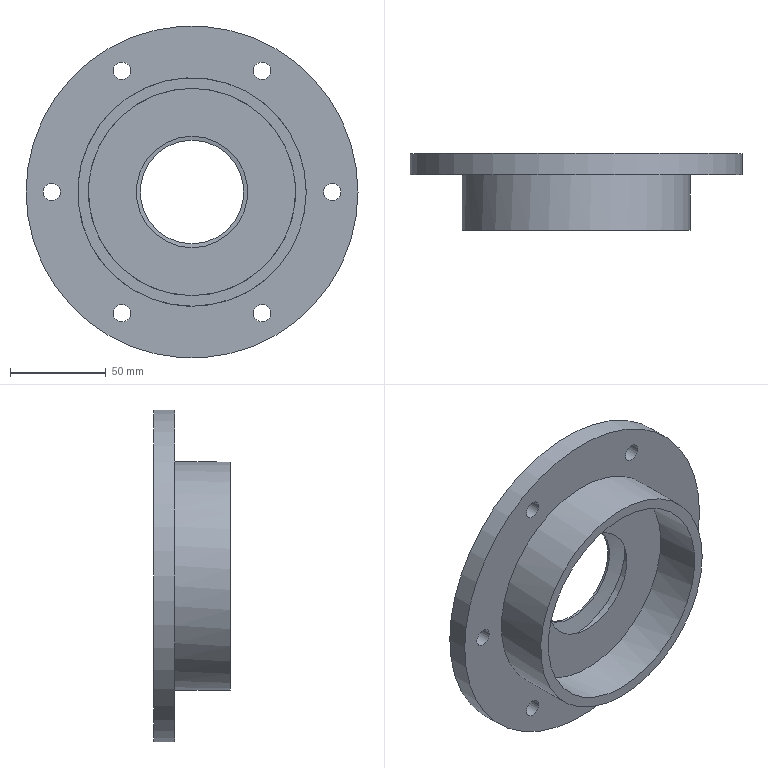Part | NX | features DATUM_CSYS 10, HOLE PACKAGE 10, SIMPLE HOLE 10, SKETCH 9, EXTRACT_DATUM_AXIS 6, EXTRACT_FACE 6, Instance Feature 5, EXTRUDE 2, DELETE FACE 1, OFFSET_REGION 1, Pattern Feature 1, SWP104 1 | 1 solid | 19 faces | box 173 x 40 x 173 mm | volume 270737 mm3 | cylinder 12 | plane 5 | cone 2 | commonest cylinder face diameters 9 x6 54 x1 74 x1 108 x1 114 x1 119 x1
STEP:
#1=CARTESIAN_POINT('',(0.,-15.,54.));
#2=VERTEX_POINT('',#1);
#3=CARTESIAN_POINT('',(0.,-15.,0.));
#4=DIRECTION('',(0.,1.,0.));
#5=DIRECTION('',(0.,0.,1.));
#6=AXIS2_PLACEMENT_3D('',#3,#4,#5);
#7=CIRCLE('',#6,54.);
#8=EDGE_CURVE('',#2,#2,#7,.F.);
#9=ORIENTED_EDGE('',*,*,#8,.T.);
#10=EDGE_LOOP('',(#9));
#11=FACE_BOUND('',#10,.T.);
#12=CARTESIAN_POINT('',(0.,-15.,29.059));
#13=VERTEX_POINT('',#12);
#14=CARTESIAN_POINT('',(0.,-15.,0.));
#15=DIRECTION('',(0.,1.,0.));
#16=DIRECTION('',(0.,0.,1.));
#17=AXIS2_PLACEMENT_3D('',#14,#15,#16);
#18=CIRCLE('',#17,29.059);
#19=EDGE_CURVE('',#13,#13,#18,.F.);
#20=ORIENTED_EDGE('',*,*,#19,.F.);
#21=EDGE_LOOP('',(#20));
#22=FACE_BOUND('',#21,.T.);
#23=CARTESIAN_POINT('',(0.,-15.,0.));
#24=DIRECTION('',(0.,1.,0.));
#25=DIRECTION('',(0.,0.,1.));
#26=AXIS2_PLACEMENT_3D('',#23,#24,#25);
#27=PLANE('',#26);
#28=ADVANCED_FACE('',(#11,#22),#27,.F.);
#29=CARTESIAN_POINT('',(86.5,-11.,0.));
#30=VERTEX_POINT('',#29);
#31=CARTESIAN_POINT('',(0.,-11.,0.));
#32=DIRECTION('',(0.,-1.,0.));
#33=DIRECTION('',(1.,0.,0.));
#34=AXIS2_PLACEMENT_3D('',#31,#32,#33);
#35=CIRCLE('',#34,86.5);
#36=EDGE_CURVE('',#30,#30,#35,.T.);
#37=ORIENTED_EDGE('',*,*,#36,.F.);
#38=EDGE_LOOP('',(#37));
#39=FACE_BOUND('',#38,.T.);
#40=CARTESIAN_POINT('',(86.5,0.,0.));
#41=VERTEX_POINT('',#40);
#42=CARTESIAN_POINT('',(0.,0.,0.));
#43=DIRECTION('',(0.,-1.,0.));
#44=DIRECTION('',(1.,0.,0.));
#45=AXIS2_PLACEMENT_3D('',#42,#43,#44);
#46=CIRCLE('',#45,86.5);
#47=EDGE_CURVE('',#41,#41,#46,.T.);
#48=ORIENTED_EDGE('',*,*,#47,.T.);
#49=EDGE_LOOP('',(#48));
#50=FACE_BOUND('',#49,.T.);
#51=CARTESIAN_POINT('',(0.,-11.,0.));
#52=DIRECTION('',(0.,1.,0.));
#53=DIRECTION('',(0.,0.,1.));
#54=AXIS2_PLACEMENT_3D('',#51,#52,#53);
#55=CYLINDRICAL_SURFACE('',#54,86.5);
#56=ADVANCED_FACE('',(#39,#50),#55,.T.);
#57=CARTESIAN_POINT('',(-36.5,-11.,-67.72));
#58=VERTEX_POINT('',#57);
#59=CARTESIAN_POINT('',(-36.5,-11.,-63.22));
#60=DIRECTION('',(0.,-1.,0.));
#61=DIRECTION('',(0.,0.,-1.));
#62=AXIS2_PLACEMENT_3D('',#59,#60,#61);
#63=CIRCLE('',#62,4.5);
#64=EDGE_CURVE('',#58,#58,#63,.T.);
#65=ORIENTED_EDGE('',*,*,#64,.F.);
#66=EDGE_LOOP('',(#65));
#67=FACE_BOUND('',#66,.T.);
#68=CARTESIAN_POINT('',(36.5,-11.,-67.72));
#69=VERTEX_POINT('',#68);
#70=CARTESIAN_POINT('',(36.5,-11.,-63.22));
#71=DIRECTION('',(0.,-1.,0.));
#72=DIRECTION('',(0.,0.,-1.));
#73=AXIS2_PLACEMENT_3D('',#70,#71,#72);
#74=CIRCLE('',#73,4.5);
#75=EDGE_CURVE('',#69,#69,#74,.T.);
#76=ORIENTED_EDGE('',*,*,#75,.F.);
#77=EDGE_LOOP('',(#76));
#78=FACE_BOUND('',#77,.T.);
#79=CARTESIAN_POINT('',(73.,-11.,-4.5));
#80=VERTEX_POINT('',#79);
#81=CARTESIAN_POINT('',(73.,-11.,0.));
#82=DIRECTION('',(0.,-1.,0.));
#83=DIRECTION('',(0.,0.,-1.));
#84=AXIS2_PLACEMENT_3D('',#81,#82,#83);
#85=CIRCLE('',#84,4.5);
#86=EDGE_CURVE('',#80,#80,#85,.T.);
#87=ORIENTED_EDGE('',*,*,#86,.F.);
#88=EDGE_LOOP('',(#87));
#89=FACE_BOUND('',#88,.T.);
#90=CARTESIAN_POINT('',(36.5,-11.,58.72));
#91=VERTEX_POINT('',#90);
#92=CARTESIAN_POINT('',(36.5,-11.,63.22));
#93=DIRECTION('',(0.,-1.,0.));
#94=DIRECTION('',(0.,0.,-1.));
#95=AXIS2_PLACEMENT_3D('',#92,#93,#94);
#96=CIRCLE('',#95,4.5);
#97=EDGE_CURVE('',#91,#91,#96,.T.);
#98=ORIENTED_EDGE('',*,*,#97,.F.);
#99=EDGE_LOOP('',(#98));
#100=FACE_BOUND('',#99,.T.);
#101=CARTESIAN_POINT('',(-36.5,-11.,58.72));
#102=VERTEX_POINT('',#101);
#103=CARTESIAN_POINT('',(-36.5,-11.,63.22));
#104=DIRECTION('',(0.,-1.,0.));
#105=DIRECTION('',(0.,0.,-1.));
#106=AXIS2_PLACEMENT_3D('',#103,#104,#105);
#107=CIRCLE('',#106,4.5);
#108=EDGE_CURVE('',#102,#102,#107,.T.);
#109=ORIENTED_EDGE('',*,*,#108,.F.);
#110=EDGE_LOOP('',(#109));
#111=FACE_BOUND('',#110,.T.);
#112=CARTESIAN_POINT('',(-73.,-11.,-4.5));
#113=VERTEX_POINT('',#112);
#114=CARTESIAN_POINT('',(-73.,-11.,0.));
#115=DIRECTION('',(0.,-1.,0.));
#116=DIRECTION('',(0.,0.,-1.));
#117=AXIS2_PLACEMENT_3D('',#114,#115,#116);
#118=CIRCLE('',#117,4.5);
#119=EDGE_CURVE('',#113,#113,#118,.T.);
#120=ORIENTED_EDGE('',*,*,#119,.F.);
#121=EDGE_LOOP('',(#120));
#122=FACE_BOUND('',#121,.T.);
#123=CARTESIAN_POINT('',(59.5,-11.,0.));
#124=VERTEX_POINT('',#123);
#125=CARTESIAN_POINT('',(0.,-11.,0.));
#126=DIRECTION('',(0.,-1.,0.));
#127=DIRECTION('',(1.,0.,0.));
#128=AXIS2_PLACEMENT_3D('',#125,#126,#127);
#129=CIRCLE('',#128,59.5);
#130=EDGE_CURVE('',#124,#124,#129,.T.);
#131=ORIENTED_EDGE('',*,*,#130,.F.);
#132=EDGE_LOOP('',(#131));
#133=FACE_BOUND('',#132,.T.);
#134=ORIENTED_EDGE('',*,*,#36,.T.);
#135=EDGE_LOOP('',(#134));
#136=FACE_BOUND('',#135,.T.);
#137=CARTESIAN_POINT('',(0.,-11.,0.));
#138=DIRECTION('',(0.,-1.,0.));
#139=DIRECTION('',(0.,0.,-1.));
#140=AXIS2_PLACEMENT_3D('',#137,#138,#139);
#141=PLANE('',#140);
#142=ADVANCED_FACE('',(#67,#78,#89,#100,#111,#122,#133,#136),#141,.T.);
#143=CARTESIAN_POINT('',(-36.5,0.,-67.72));
#144=VERTEX_POINT('',#143);
#145=CARTESIAN_POINT('',(-36.5,0.,-63.22));
#146=DIRECTION('',(0.,-1.,0.));
#147=DIRECTION('',(0.,0.,-1.));
#148=AXIS2_PLACEMENT_3D('',#145,#146,#147);
#149=CIRCLE('',#148,4.5);
#150=EDGE_CURVE('',#144,#144,#149,.T.);
#151=ORIENTED_EDGE('',*,*,#150,.T.);
#152=EDGE_LOOP('',(#151));
#153=FACE_BOUND('',#152,.T.);
#154=CARTESIAN_POINT('',(36.5,0.,-67.72));
#155=VERTEX_POINT('',#154);
#156=CARTESIAN_POINT('',(36.5,0.,-63.22));
#157=DIRECTION('',(0.,-1.,0.));
#158=DIRECTION('',(0.,0.,-1.));
#159=AXIS2_PLACEMENT_3D('',#156,#157,#158);
#160=CIRCLE('',#159,4.5);
#161=EDGE_CURVE('',#155,#155,#160,.T.);
#162=ORIENTED_EDGE('',*,*,#161,.T.);
#163=EDGE_LOOP('',(#162));
#164=FACE_BOUND('',#163,.T.);
#165=CARTESIAN_POINT('',(73.,0.,-4.5));
#166=VERTEX_POINT('',#165);
#167=CARTESIAN_POINT('',(73.,0.,0.));
#168=DIRECTION('',(0.,-1.,0.));
#169=DIRECTION('',(0.,0.,-1.));
#170=AXIS2_PLACEMENT_3D('',#167,#168,#169);
#171=CIRCLE('',#170,4.5);
#172=EDGE_CURVE('',#166,#166,#171,.T.);
#173=ORIENTED_EDGE('',*,*,#172,.T.);
#174=EDGE_LOOP('',(#173));
#175=FACE_BOUND('',#174,.T.);
#176=CARTESIAN_POINT('',(36.5,0.,58.72));
#177=VERTEX_POINT('',#176);
#178=CARTESIAN_POINT('',(36.5,0.,63.22));
#179=DIRECTION('',(0.,-1.,0.));
#180=DIRECTION('',(0.,0.,-1.));
#181=AXIS2_PLACEMENT_3D('',#178,#179,#180);
#182=CIRCLE('',#181,4.5);
#183=EDGE_CURVE('',#177,#177,#182,.T.);
#184=ORIENTED_EDGE('',*,*,#183,.T.);
#185=EDGE_LOOP('',(#184));
#186=FACE_BOUND('',#185,.T.);
#187=CARTESIAN_POINT('',(-36.5,0.,58.72));
#188=VERTEX_POINT('',#187);
#189=CARTESIAN_POINT('',(-36.5,0.,63.22));
#190=DIRECTION('',(0.,-1.,0.));
#191=DIRECTION('',(0.,0.,-1.));
#192=AXIS2_PLACEMENT_3D('',#189,#190,#191);
#193=CIRCLE('',#192,4.5);
#194=EDGE_CURVE('',#188,#188,#193,.T.);
#195=ORIENTED_EDGE('',*,*,#194,.T.);
#196=EDGE_LOOP('',(#195));
#197=FACE_BOUND('',#196,.T.);
#198=CARTESIAN_POINT('',(-73.,0.,-4.5));
#199=VERTEX_POINT('',#198);
#200=CARTESIAN_POINT('',(-73.,0.,0.));
#201=DIRECTION('',(0.,-1.,0.));
#202=DIRECTION('',(0.,0.,-1.));
#203=AXIS2_PLACEMENT_3D('',#200,#201,#202);
#204=CIRCLE('',#203,4.5);
#205=EDGE_CURVE('',#199,#199,#204,.T.);
#206=ORIENTED_EDGE('',*,*,#205,.T.);
#207=EDGE_LOOP('',(#206));
#208=FACE_BOUND('',#207,.T.);
#209=CARTESIAN_POINT('',(0.,0.,-57.));
#210=VERTEX_POINT('',#209);
#211=CARTESIAN_POINT('',(0.,0.,0.));
#212=DIRECTION('',(0.,-1.,0.));
#213=DIRECTION('',(0.,0.,-1.));
#214=AXIS2_PLACEMENT_3D('',#211,#212,#213);
#215=CIRCLE('',#214,57.);
#216=EDGE_CURVE('',#210,#210,#215,.T.);
#217=ORIENTED_EDGE('',*,*,#216,.T.);
#218=EDGE_LOOP('',(#217));
#219=FACE_BOUND('',#218,.T.);
#220=ORIENTED_EDGE('',*,*,#47,.F.);
#221=EDGE_LOOP('',(#220));
#222=FACE_BOUND('',#221,.T.);
#223=CARTESIAN_POINT('',(0.,0.,0.));
#224=DIRECTION('',(0.,-1.,0.));
#225=DIRECTION('',(0.,0.,-1.));
#226=AXIS2_PLACEMENT_3D('',#223,#224,#225);
#227=PLANE('',#226);
#228=ADVANCED_FACE('',(#153,#164,#175,#186,#197,#208,#219,#222),#227,.F.);
#229=CARTESIAN_POINT('',(0.,-40.,-59.5));
#230=VERTEX_POINT('',#229);
#231=CARTESIAN_POINT('',(0.,-40.,0.));
#232=DIRECTION('',(0.,-1.,0.));
#233=DIRECTION('',(0.,0.,-1.));
#234=AXIS2_PLACEMENT_3D('',#231,#232,#233);
#235=CIRCLE('',#234,59.5);
#236=EDGE_CURVE('',#230,#230,#235,.T.);
#237=ORIENTED_EDGE('',*,*,#236,.F.);
#238=EDGE_LOOP('',(#237));
#239=FACE_BOUND('',#238,.T.);
#240=ORIENTED_EDGE('',*,*,#130,.T.);
#241=EDGE_LOOP('',(#240));
#242=FACE_BOUND('',#241,.T.);
#243=CARTESIAN_POINT('',(0.,-35.,0.));
#244=DIRECTION('',(0.,1.,0.));
#245=DIRECTION('',(0.,0.,1.));
#246=AXIS2_PLACEMENT_3D('',#243,#244,#245);
#247=CYLINDRICAL_SURFACE('',#246,59.5);
#248=ADVANCED_FACE('',(#239,#242),#247,.T.);
#249=CARTESIAN_POINT('',(0.,-40.,-54.));
#250=VERTEX_POINT('',#249);
#251=CARTESIAN_POINT('',(0.,-40.,0.));
#252=DIRECTION('',(0.,-1.,0.));
#253=DIRECTION('',(0.,0.,-1.));
#254=AXIS2_PLACEMENT_3D('',#251,#252,#253);
#255=CIRCLE('',#254,54.);
#256=EDGE_CURVE('',#250,#250,#255,.F.);
#257=ORIENTED_EDGE('',*,*,#256,.T.);
#258=EDGE_LOOP('',(#257));
#259=FACE_BOUND('',#258,.T.);
#260=ORIENTED_EDGE('',*,*,#236,.T.);
#261=EDGE_LOOP('',(#260));
#262=FACE_BOUND('',#261,.T.);
#263=CARTESIAN_POINT('',(0.,-40.,0.));
#264=DIRECTION('',(0.,-1.,0.));
#265=DIRECTION('',(0.,0.,-1.));
#266=AXIS2_PLACEMENT_3D('',#263,#264,#265);
#267=PLANE('',#266);
#268=ADVANCED_FACE('',(#259,#262),#267,.T.);
#269=ORIENTED_EDGE('',*,*,#8,.F.);
#270=EDGE_LOOP('',(#269));
#271=FACE_BOUND('',#270,.T.);
#272=ORIENTED_EDGE('',*,*,#256,.F.);
#273=EDGE_LOOP('',(#272));
#274=FACE_BOUND('',#273,.T.);
#275=CARTESIAN_POINT('',(0.,-35.,0.));
#276=DIRECTION('',(0.,1.,0.));
#277=DIRECTION('',(0.,0.,1.));
#278=AXIS2_PLACEMENT_3D('',#275,#276,#277);
#279=CYLINDRICAL_SURFACE('',#278,54.);
#280=ADVANCED_FACE('',(#271,#274),#279,.F.);
#281=CARTESIAN_POINT('',(0.,-3.,-27.));
#282=VERTEX_POINT('',#281);
#283=CARTESIAN_POINT('',(0.,-3.,0.));
#284=DIRECTION('',(0.,-1.,0.));
#285=DIRECTION('',(0.,0.,-1.));
#286=AXIS2_PLACEMENT_3D('',#283,#284,#285);
#287=CIRCLE('',#286,27.);
#288=EDGE_CURVE('',#282,#282,#287,.T.);
#289=ORIENTED_EDGE('',*,*,#288,.T.);
#290=EDGE_LOOP('',(#289));
#291=FACE_BOUND('',#290,.T.);
#292=CARTESIAN_POINT('',(0.,-3.,-57.));
#293=VERTEX_POINT('',#292);
#294=CARTESIAN_POINT('',(0.,-3.,0.));
#295=DIRECTION('',(0.,-1.,0.));
#296=DIRECTION('',(0.,0.,-1.));
#297=AXIS2_PLACEMENT_3D('',#294,#295,#296);
#298=CIRCLE('',#297,57.);
#299=EDGE_CURVE('',#293,#293,#298,.F.);
#300=ORIENTED_EDGE('',*,*,#299,.T.);
#301=EDGE_LOOP('',(#300));
#302=FACE_BOUND('',#301,.T.);
#303=CARTESIAN_POINT('',(0.,-3.,0.));
#304=DIRECTION('',(0.,-1.,0.));
#305=DIRECTION('',(0.,0.,-1.));
#306=AXIS2_PLACEMENT_3D('',#303,#304,#305);
#307=PLANE('',#306);
#308=ADVANCED_FACE('',(#291,#302),#307,.F.);
#309=ORIENTED_EDGE('',*,*,#299,.F.);
#310=EDGE_LOOP('',(#309));
#311=FACE_BOUND('',#310,.T.);
#312=ORIENTED_EDGE('',*,*,#216,.F.);
#313=EDGE_LOOP('',(#312));
#314=FACE_BOUND('',#313,.T.);
#315=CARTESIAN_POINT('',(0.,0.,0.));
#316=DIRECTION('',(0.,-1.,0.));
#317=DIRECTION('',(0.,0.,-1.));
#318=AXIS2_PLACEMENT_3D('',#315,#316,#317);
#319=CYLINDRICAL_SURFACE('',#318,57.);
#320=ADVANCED_FACE('',(#311,#314),#319,.F.);
#321=ORIENTED_EDGE('',*,*,#119,.T.);
#322=EDGE_LOOP('',(#321));
#323=FACE_BOUND('',#322,.T.);
#324=ORIENTED_EDGE('',*,*,#205,.F.);
#325=EDGE_LOOP('',(#324));
#326=FACE_BOUND('',#325,.T.);
#327=CARTESIAN_POINT('',(-73.,0.,0.));
#328=DIRECTION('',(0.,-1.,0.));
#329=DIRECTION('',(0.,0.,-1.));
#330=AXIS2_PLACEMENT_3D('',#327,#328,#329);
#331=CYLINDRICAL_SURFACE('',#330,4.5);
#332=ADVANCED_FACE('',(#323,#326),#331,.F.);
#333=ORIENTED_EDGE('',*,*,#108,.T.);
#334=EDGE_LOOP('',(#333));
#335=FACE_BOUND('',#334,.T.);
#336=ORIENTED_EDGE('',*,*,#194,.F.);
#337=EDGE_LOOP('',(#336));
#338=FACE_BOUND('',#337,.T.);
#339=CARTESIAN_POINT('',(-36.5,0.,63.22));
#340=DIRECTION('',(0.,-1.,0.));
#341=DIRECTION('',(0.,0.,-1.));
#342=AXIS2_PLACEMENT_3D('',#339,#340,#341);
#343=CYLINDRICAL_SURFACE('',#342,4.5);
#344=ADVANCED_FACE('',(#335,#338),#343,.F.);
#345=ORIENTED_EDGE('',*,*,#97,.T.);
#346=EDGE_LOOP('',(#345));
#347=FACE_BOUND('',#346,.T.);
#348=ORIENTED_EDGE('',*,*,#183,.F.);
#349=EDGE_LOOP('',(#348));
#350=FACE_BOUND('',#349,.T.);
#351=CARTESIAN_POINT('',(36.5,0.,63.22));
#352=DIRECTION('',(0.,-1.,0.));
#353=DIRECTION('',(0.,0.,-1.));
#354=AXIS2_PLACEMENT_3D('',#351,#352,#353);
#355=CYLINDRICAL_SURFACE('',#354,4.5);
#356=ADVANCED_FACE('',(#347,#350),#355,.F.);
#357=ORIENTED_EDGE('',*,*,#86,.T.);
#358=EDGE_LOOP('',(#357));
#359=FACE_BOUND('',#358,.T.);
#360=ORIENTED_EDGE('',*,*,#172,.F.);
#361=EDGE_LOOP('',(#360));
#362=FACE_BOUND('',#361,.T.);
#363=CARTESIAN_POINT('',(73.,0.,0.));
#364=DIRECTION('',(0.,-1.,0.));
#365=DIRECTION('',(0.,0.,-1.));
#366=AXIS2_PLACEMENT_3D('',#363,#364,#365);
#367=CYLINDRICAL_SURFACE('',#366,4.5);
#368=ADVANCED_FACE('',(#359,#362),#367,.F.);
#369=ORIENTED_EDGE('',*,*,#75,.T.);
#370=EDGE_LOOP('',(#369));
#371=FACE_BOUND('',#370,.T.);
#372=ORIENTED_EDGE('',*,*,#161,.F.);
#373=EDGE_LOOP('',(#372));
#374=FACE_BOUND('',#373,.T.);
#375=CARTESIAN_POINT('',(36.5,0.,-63.22));
#376=DIRECTION('',(0.,-1.,0.));
#377=DIRECTION('',(0.,0.,-1.));
#378=AXIS2_PLACEMENT_3D('',#375,#376,#377);
#379=CYLINDRICAL_SURFACE('',#378,4.5);
#380=ADVANCED_FACE('',(#371,#374),#379,.F.);
#381=ORIENTED_EDGE('',*,*,#64,.T.);
#382=EDGE_LOOP('',(#381));
#383=FACE_BOUND('',#382,.T.);
#384=ORIENTED_EDGE('',*,*,#150,.F.);
#385=EDGE_LOOP('',(#384));
#386=FACE_BOUND('',#385,.T.);
#387=CARTESIAN_POINT('',(-36.5,0.,-63.22));
#388=DIRECTION('',(0.,-1.,0.));
#389=DIRECTION('',(0.,0.,-1.));
#390=AXIS2_PLACEMENT_3D('',#387,#388,#389);
#391=CYLINDRICAL_SURFACE('',#390,4.5);
#392=ADVANCED_FACE('',(#383,#386),#391,.F.);
#393=CARTESIAN_POINT('',(0.,-13.742,-37.));
#394=VERTEX_POINT('',#393);
#395=CARTESIAN_POINT('',(0.,-13.742,0.));
#396=DIRECTION('',(0.,-1.,0.));
#397=DIRECTION('',(0.,0.,-1.));
#398=AXIS2_PLACEMENT_3D('',#395,#396,#397);
#399=CIRCLE('',#398,37.);
#400=EDGE_CURVE('',#394,#394,#399,.F.);
#401=ORIENTED_EDGE('',*,*,#400,.T.);
#402=EDGE_LOOP('',(#401));
#403=FACE_BOUND('',#402,.T.);
#404=ORIENTED_EDGE('',*,*,#19,.T.);
#405=EDGE_LOOP('',(#404));
#406=FACE_BOUND('',#405,.T.);
#407=CARTESIAN_POINT('',(0.,-13.742,0.));
#408=DIRECTION('',(0.,1.,0.));
#409=DIRECTION('',(0.,0.,1.));
#410=AXIS2_PLACEMENT_3D('',#407,#408,#409);
#411=CONICAL_SURFACE('',#410,37.,1.414);
#412=ADVANCED_FACE('',(#403,#406),#411,.F.);
#413=CARTESIAN_POINT('',(0.,-4.158,-27.));
#414=VERTEX_POINT('',#413);
#415=CARTESIAN_POINT('',(0.,-4.158,0.));
#416=DIRECTION('',(0.,-1.,0.));
#417=DIRECTION('',(0.,0.,-1.));
#418=AXIS2_PLACEMENT_3D('',#415,#416,#417);
#419=CIRCLE('',#418,27.);
#420=EDGE_CURVE('',#414,#414,#419,.T.);
#421=ORIENTED_EDGE('',*,*,#420,.F.);
#422=EDGE_LOOP('',(#421));
#423=FACE_BOUND('',#422,.T.);
#424=CARTESIAN_POINT('',(0.,-5.742,-37.));
#425=VERTEX_POINT('',#424);
#426=CARTESIAN_POINT('',(0.,-5.742,0.));
#427=DIRECTION('',(0.,-1.,0.));
#428=DIRECTION('',(0.,0.,-1.));
#429=AXIS2_PLACEMENT_3D('',#426,#427,#428);
#430=CIRCLE('',#429,37.);
#431=EDGE_CURVE('',#425,#425,#430,.F.);
#432=ORIENTED_EDGE('',*,*,#431,.F.);
#433=EDGE_LOOP('',(#432));
#434=FACE_BOUND('',#433,.T.);
#435=CARTESIAN_POINT('',(0.,-4.,0.));
#436=DIRECTION('',(0.,-1.,0.));
#437=DIRECTION('',(0.,0.,-1.));
#438=AXIS2_PLACEMENT_3D('',#435,#436,#437);
#439=CONICAL_SURFACE('',#438,26.,1.414);
#440=ADVANCED_FACE('',(#423,#434),#439,.F.);
#441=ORIENTED_EDGE('',*,*,#400,.F.);
#442=EDGE_LOOP('',(#441));
#443=FACE_BOUND('',#442,.T.);
#444=ORIENTED_EDGE('',*,*,#431,.T.);
#445=EDGE_LOOP('',(#444));
#446=FACE_BOUND('',#445,.T.);
#447=CARTESIAN_POINT('',(0.,0.,0.));
#448=DIRECTION('',(0.,-1.,0.));
#449=DIRECTION('',(0.,0.,-1.));
#450=AXIS2_PLACEMENT_3D('',#447,#448,#449);
#451=CYLINDRICAL_SURFACE('',#450,37.);
#452=ADVANCED_FACE('',(#443,#446),#451,.F.);
#453=ORIENTED_EDGE('',*,*,#420,.T.);
#454=EDGE_LOOP('',(#453));
#455=FACE_BOUND('',#454,.T.);
#456=ORIENTED_EDGE('',*,*,#288,.F.);
#457=EDGE_LOOP('',(#456));
#458=FACE_BOUND('',#457,.T.);
#459=CARTESIAN_POINT('',(0.,0.,0.));
#460=DIRECTION('',(0.,-1.,0.));
#461=DIRECTION('',(0.,0.,-1.));
#462=AXIS2_PLACEMENT_3D('',#459,#460,#461);
#463=CYLINDRICAL_SURFACE('',#462,27.);
#464=ADVANCED_FACE('',(#455,#458),#463,.F.);
#465=CLOSED_SHELL('',(#28,#56,#142,#228,#248,#268,#280,#308,#320,#332,#344,#356,#368,#380,#392,#412,#440,#452,#464));
#466=MANIFOLD_SOLID_BREP('',#465);
#467=(LENGTH_UNIT()NAMED_UNIT(*)SI_UNIT(.MILLI.,.METRE.));
#468=UNCERTAINTY_MEASURE_WITH_UNIT(LENGTH_MEASURE(0.00001),#467,'','');
#469=(NAMED_UNIT(*)PLANE_ANGLE_UNIT()SI_UNIT($,.RADIAN.));
#470=(NAMED_UNIT(*)SI_UNIT($,.STERADIAN.)SOLID_ANGLE_UNIT());
#471=(GEOMETRIC_REPRESENTATION_CONTEXT(3)GLOBAL_UNCERTAINTY_ASSIGNED_CONTEXT((#468))GLOBAL_UNIT_ASSIGNED_CONTEXT((#467,#469,#470))REPRESENTATION_CONTEXT('',''));
#472=ADVANCED_BREP_SHAPE_REPRESENTATION('',(#466),#471);